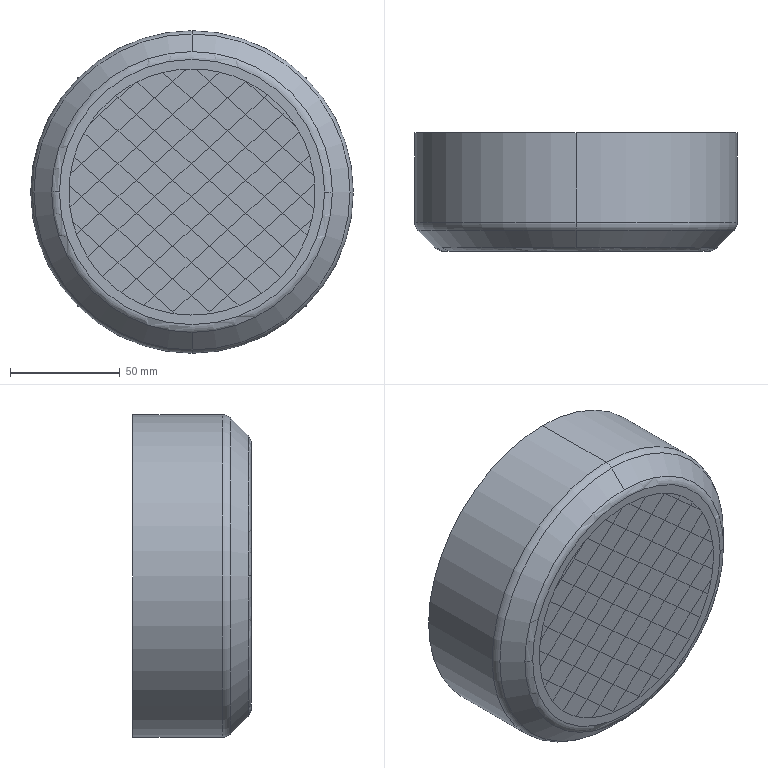Part | SolidWorks | features BaseBody 1 | 1 solid | 113 faces | box 147 x 54 x 147 mm | volume 56536 mm3 | plane 101 | torus 4 | cone 4 | cylinder 4 | commonest cylinder face diameters 144 x2 147 x2